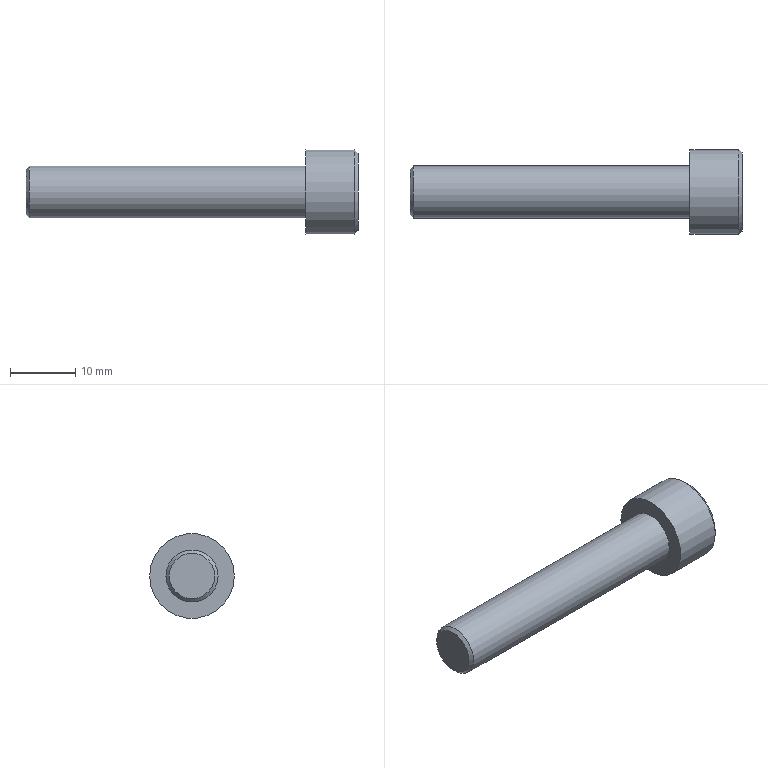Part | NX | features CHAMFER 6, BREP 2, solid 2, SUBTRACT 1 | 1 solid | 36 faces | box 51 x 13 x 13 mm | volume 3079 mm3 | plane 23 | spline 9 | cylinder 2 | cone 2 | commonest cylinder face diameters 8 x1 13 x1
STEP:
#1=CARTESIAN_POINT('',(260.,-279.45,211.002));
#2=VERTEX_POINT('',#1);
#3=CARTESIAN_POINT('',(260.,-279.625,211.545));
#4=VERTEX_POINT('',#3);
#5=CARTESIAN_POINT('',(260.,-279.45,211.002));
#6=CARTESIAN_POINT('',(260.,-279.385,211.002));
#7=CARTESIAN_POINT('',(260.,-279.327,211.016));
#8=CARTESIAN_POINT('',(260.,-279.225,211.073));
#9=CARTESIAN_POINT('',(260.,-279.185,211.113));
#10=CARTESIAN_POINT('',(260.,-279.128,211.215));
#11=CARTESIAN_POINT('',(260.,-279.114,211.272));
#12=CARTESIAN_POINT('',(260.,-279.114,211.377));
#13=CARTESIAN_POINT('',(260.,-279.121,211.418));
#14=CARTESIAN_POINT('',(260.,-279.15,211.497));
#15=CARTESIAN_POINT('',(260.,-279.171,211.531));
#16=CARTESIAN_POINT('',(260.,-279.224,211.589));
#17=CARTESIAN_POINT('',(260.,-279.256,211.611));
#18=CARTESIAN_POINT('',(260.,-279.327,211.643));
#19=CARTESIAN_POINT('',(260.,-279.366,211.651));
#20=CARTESIAN_POINT('',(260.,-279.452,211.651));
#21=CARTESIAN_POINT('',(260.,-279.491,211.642));
#22=CARTESIAN_POINT('',(260.,-279.562,211.608));
#23=CARTESIAN_POINT('',(260.,-279.595,211.581));
#24=CARTESIAN_POINT('',(260.,-279.625,211.545));
#25=B_SPLINE_CURVE_WITH_KNOTS('',3,(#5,#6,#7,#8,#9,#10,#11,#12,#13,#14,#15,#16,#17,#18,#19,#20,#21,#22,#23,#24),.UNSPECIFIED.,.F.,.F.,(4,2,2,2,2,2,2,2,2,4),(0.,0.02844,0.05688,0.08532,0.1049,0.1245,0.144,0.1636,0.184,0.2044),.UNSPECIFIED.);
#26=EDGE_CURVE('',#2,#4,#25,.T.);
#27=ORIENTED_EDGE('',*,*,#26,.F.);
#28=CARTESIAN_POINT('',(260.,-279.314,211.783));
#29=VERTEX_POINT('',#28);
#30=CARTESIAN_POINT('',(260.,-279.314,211.783));
#31=CARTESIAN_POINT('',(260.,-279.306,211.762));
#32=CARTESIAN_POINT('',(260.,-279.294,211.746));
#33=CARTESIAN_POINT('',(260.,-279.262,211.722));
#34=CARTESIAN_POINT('',(260.,-279.245,211.716));
#35=CARTESIAN_POINT('',(260.,-279.205,211.716));
#36=CARTESIAN_POINT('',(260.,-279.188,211.724));
#37=CARTESIAN_POINT('',(260.,-279.16,211.754));
#38=CARTESIAN_POINT('',(260.,-279.154,211.77));
#39=CARTESIAN_POINT('',(260.,-279.154,211.818));
#40=CARTESIAN_POINT('',(260.,-279.164,211.85));
#41=CARTESIAN_POINT('',(260.,-279.208,211.915));
#42=CARTESIAN_POINT('',(260.,-279.241,211.943));
#43=CARTESIAN_POINT('',(260.,-279.327,211.987));
#44=CARTESIAN_POINT('',(260.,-279.377,211.998));
#45=CARTESIAN_POINT('',(260.,-279.493,211.998));
#46=CARTESIAN_POINT('',(260.,-279.545,211.987));
#47=CARTESIAN_POINT('',(260.,-279.637,211.943));
#48=CARTESIAN_POINT('',(260.,-279.676,211.91));
#49=CARTESIAN_POINT('',(260.,-279.741,211.823));
#50=CARTESIAN_POINT('',(260.,-279.766,211.769));
#51=CARTESIAN_POINT('',(260.,-279.8,211.637));
#52=CARTESIAN_POINT('',(260.,-279.809,211.562));
#53=CARTESIAN_POINT('',(260.,-279.809,211.375));
#54=CARTESIAN_POINT('',(260.,-279.795,211.288));
#55=CARTESIAN_POINT('',(260.,-279.738,211.146));
#56=CARTESIAN_POINT('',(260.,-279.696,211.093));
#57=CARTESIAN_POINT('',(260.,-279.588,211.02));
#58=CARTESIAN_POINT('',(260.,-279.524,211.002));
#59=CARTESIAN_POINT('',(260.,-279.45,211.002));
#60=B_SPLINE_CURVE_WITH_KNOTS('',3,(#30,#31,#32,#33,#34,#35,#36,#37,#38,#39,#40,#41,#42,#43,#44,#45,#46,#47,#48,#49,#50,#51,#52,#53,#54,#55,#56,#57,#58,#59),.UNSPECIFIED.,.F.,.F.,(4,2,2,2,2,2,2,2,2,2,2,2,2,2,4),(0.3727,0.3977,0.4227,0.4513,0.4798,0.5272,0.5745,0.6219,0.6711,0.7203,0.7695,0.8188,0.8792,0.9396,1.),.UNSPECIFIED.);
#61=EDGE_CURVE('',#29,#2,#60,.T.);
#62=ORIENTED_EDGE('',*,*,#61,.F.);
#63=CARTESIAN_POINT('',(260.,-279.568,211.796));
#64=VERTEX_POINT('',#63);
#65=CARTESIAN_POINT('',(260.,-279.568,211.796));
#66=CARTESIAN_POINT('',(260.,-279.552,211.819));
#67=CARTESIAN_POINT('',(260.,-279.532,211.837));
#68=CARTESIAN_POINT('',(260.,-279.486,211.864));
#69=CARTESIAN_POINT('',(260.,-279.463,211.871));
#70=CARTESIAN_POINT('',(260.,-279.41,211.871));
#71=CARTESIAN_POINT('',(260.,-279.384,211.863));
#72=CARTESIAN_POINT('',(260.,-279.34,211.831));
#73=CARTESIAN_POINT('',(260.,-279.324,211.809));
#74=CARTESIAN_POINT('',(260.,-279.314,211.783));
#75=B_SPLINE_CURVE_WITH_KNOTS('',3,(#65,#66,#67,#68,#69,#70,#71,#72,#73,#74),.UNSPECIFIED.,.F.,.F.,(4,2,2,2,4),(0.2569,0.2827,0.3085,0.3406,0.3727),.UNSPECIFIED.);
#76=EDGE_CURVE('',#64,#29,#75,.T.);
#77=ORIENTED_EDGE('',*,*,#76,.F.);
#78=CARTESIAN_POINT('',(260.,-279.625,211.545));
#79=CARTESIAN_POINT('',(260.,-279.619,211.666));
#80=CARTESIAN_POINT('',(260.,-279.6,211.749));
#81=CARTESIAN_POINT('',(260.,-279.568,211.796));
#82=B_SPLINE_CURVE_WITH_KNOTS('',3,(#78,#79,#80,#81),.UNSPECIFIED.,.F.,.F.,(4,4),(0.2044,0.2569),.PIECEWISE_BEZIER_KNOTS.);
#83=EDGE_CURVE('',#4,#64,#82,.T.);
#84=ORIENTED_EDGE('',*,*,#83,.F.);
#85=EDGE_LOOP('',(#27,#62,#77,#84));
#86=FACE_BOUND('',#85,.T.);
#87=CARTESIAN_POINT('',(260.,-281.732,208.5));
#88=VERTEX_POINT('',#87);
#89=CARTESIAN_POINT('',(260.,-283.464,211.5));
#90=VERTEX_POINT('',#89);
#91=CARTESIAN_POINT('',(260.,-283.464,211.5));
#92=DIRECTION('',(0.,-0.5,0.866));
#93=VECTOR('',#92,1000.);
#94=LINE('',#91,#93);
#95=EDGE_CURVE('',#88,#90,#94,.T.);
#96=ORIENTED_EDGE('',*,*,#95,.F.);
#97=CARTESIAN_POINT('',(260.,-278.268,208.5));
#98=VERTEX_POINT('',#97);
#99=CARTESIAN_POINT('',(260.,-281.732,208.5));
#100=DIRECTION('',(0.,-1.,0.));
#101=VECTOR('',#100,1000.);
#102=LINE('',#99,#101);
#103=EDGE_CURVE('',#98,#88,#102,.T.);
#104=ORIENTED_EDGE('',*,*,#103,.F.);
#105=CARTESIAN_POINT('',(260.,-276.536,211.5));
#106=VERTEX_POINT('',#105);
#107=CARTESIAN_POINT('',(260.,-278.268,208.5));
#108=DIRECTION('',(0.,-0.5,-0.866));
#109=VECTOR('',#108,1000.);
#110=LINE('',#107,#109);
#111=EDGE_CURVE('',#106,#98,#110,.T.);
#112=ORIENTED_EDGE('',*,*,#111,.F.);
#113=CARTESIAN_POINT('',(260.,-278.268,214.5));
#114=VERTEX_POINT('',#113);
#115=CARTESIAN_POINT('',(260.,-276.536,211.5));
#116=DIRECTION('',(0.,0.5,-0.866));
#117=VECTOR('',#116,1000.);
#118=LINE('',#115,#117);
#119=EDGE_CURVE('',#114,#106,#118,.T.);
#120=ORIENTED_EDGE('',*,*,#119,.F.);
#121=CARTESIAN_POINT('',(260.,-281.732,214.5));
#122=VERTEX_POINT('',#121);
#123=CARTESIAN_POINT('',(260.,-278.268,214.5));
#124=DIRECTION('',(0.,1.,0.));
#125=VECTOR('',#124,1000.);
#126=LINE('',#123,#125);
#127=EDGE_CURVE('',#122,#114,#126,.T.);
#128=ORIENTED_EDGE('',*,*,#127,.F.);
#129=CARTESIAN_POINT('',(260.,-281.732,214.5));
#130=DIRECTION('',(0.,0.5,0.866));
#131=VECTOR('',#130,1000.);
#132=LINE('',#129,#131);
#133=EDGE_CURVE('',#90,#122,#132,.T.);
#134=ORIENTED_EDGE('',*,*,#133,.F.);
#135=EDGE_LOOP('',(#96,#104,#112,#120,#128,#134));
#136=FACE_BOUND('',#135,.T.);
#137=CARTESIAN_POINT('',(260.,-280.797,211.005));
#138=VERTEX_POINT('',#137);
#139=CARTESIAN_POINT('',(260.,-280.706,211.783));
#140=VERTEX_POINT('',#139);
#141=CARTESIAN_POINT('',(260.,-280.797,211.005));
#142=CARTESIAN_POINT('',(260.,-280.769,211.005));
#143=CARTESIAN_POINT('',(260.,-280.748,211.014));
#144=CARTESIAN_POINT('',(260.,-280.715,211.051));
#145=CARTESIAN_POINT('',(260.,-280.706,211.079));
#146=CARTESIAN_POINT('',(260.,-280.706,211.338));
#147=CARTESIAN_POINT('',(260.,-280.706,211.561));
#148=CARTESIAN_POINT('',(260.,-280.706,211.783));
#149=B_SPLINE_CURVE_WITH_KNOTS('',3,(#141,#142,#143,#144,#145,#146,#147,#148),.UNSPECIFIED.,.F.,.F.,(4,2,2,4),(0.,0.01767,0.03533,0.1418),.UNSPECIFIED.);
#150=EDGE_CURVE('',#138,#140,#149,.T.);
#151=ORIENTED_EDGE('',*,*,#150,.F.);
#152=CARTESIAN_POINT('',(260.,-280.561,211.859));
#153=VERTEX_POINT('',#152);
#154=CARTESIAN_POINT('',(260.,-280.561,211.859));
#155=CARTESIAN_POINT('',(260.,-280.571,211.898));
#156=CARTESIAN_POINT('',(260.,-280.58,211.925));
#157=CARTESIAN_POINT('',(260.,-280.596,211.96));
#158=CARTESIAN_POINT('',(260.,-280.608,211.972));
#159=CARTESIAN_POINT('',(260.,-280.641,211.985));
#160=CARTESIAN_POINT('',(260.,-280.667,211.988));
#161=CARTESIAN_POINT('',(260.,-280.724,211.988));
#162=CARTESIAN_POINT('',(260.,-280.744,211.988));
#163=CARTESIAN_POINT('',(260.,-280.802,211.988));
#164=CARTESIAN_POINT('',(260.,-280.831,211.981));
#165=CARTESIAN_POINT('',(260.,-280.875,211.951));
#166=CARTESIAN_POINT('',(260.,-280.886,211.923));
#167=CARTESIAN_POINT('',(260.,-280.886,211.626));
#168=CARTESIAN_POINT('',(260.,-280.886,211.371));
#169=CARTESIAN_POINT('',(260.,-280.886,211.079));
#170=CARTESIAN_POINT('',(260.,-280.878,211.051));
#171=CARTESIAN_POINT('',(260.,-280.845,211.014));
#172=CARTESIAN_POINT('',(260.,-280.823,211.005));
#173=CARTESIAN_POINT('',(260.,-280.797,211.005));
#174=B_SPLINE_CURVE_WITH_KNOTS('',3,(#154,#155,#156,#157,#158,#159,#160,#161,#162,#163,#164,#165,#166,#167,#168,#169,#170,#171,#172,#173),.UNSPECIFIED.,.F.,.F.,(4,2,2,2,2,2,2,2,2,4),(0.8075,0.8217,0.8358,0.85,0.8578,0.8723,0.8868,0.9743,0.9872,1.),.UNSPECIFIED.);
#175=EDGE_CURVE('',#153,#138,#174,.T.);
#176=ORIENTED_EDGE('',*,*,#175,.F.);
#177=CARTESIAN_POINT('',(260.,-280.42,211.33));
#178=VERTEX_POINT('',#177);
#179=CARTESIAN_POINT('',(260.,-280.435,211.385));
#180=DIRECTION('',(0.,-0.2564,0.9666));
#181=VECTOR('',#180,1000.);
#182=LINE('',#179,#181);
#183=EDGE_CURVE('',#178,#153,#182,.T.);
#184=ORIENTED_EDGE('',*,*,#183,.F.);
#185=CARTESIAN_POINT('',(260.,-280.28,211.859));
#186=VERTEX_POINT('',#185);
#187=CARTESIAN_POINT('',(260.,-280.35,211.593));
#188=DIRECTION('',(0.,-0.2564,-0.9666));
#189=VECTOR('',#188,1000.);
#190=LINE('',#187,#189);
#191=EDGE_CURVE('',#186,#178,#190,.T.);
#192=ORIENTED_EDGE('',*,*,#191,.F.);
#193=CARTESIAN_POINT('',(260.,-280.134,211.783));
#194=VERTEX_POINT('',#193);
#195=CARTESIAN_POINT('',(260.,-280.134,211.783));
#196=CARTESIAN_POINT('',(260.,-280.134,211.561));
#197=CARTESIAN_POINT('',(260.,-280.134,211.338));
#198=CARTESIAN_POINT('',(260.,-280.134,211.079));
#199=CARTESIAN_POINT('',(260.,-280.126,211.051));
#200=CARTESIAN_POINT('',(260.,-280.092,211.014));
#201=CARTESIAN_POINT('',(260.,-280.071,211.005));
#202=CARTESIAN_POINT('',(260.,-280.018,211.005));
#203=CARTESIAN_POINT('',(260.,-279.995,211.014));
#204=CARTESIAN_POINT('',(260.,-279.962,211.051));
#205=CARTESIAN_POINT('',(260.,-279.954,211.079));
#206=CARTESIAN_POINT('',(260.,-279.954,211.371));
#207=CARTESIAN_POINT('',(260.,-279.954,211.626));
#208=CARTESIAN_POINT('',(260.,-279.954,211.923));
#209=CARTESIAN_POINT('',(260.,-279.965,211.951));
#210=CARTESIAN_POINT('',(260.,-280.009,211.981));
#211=CARTESIAN_POINT('',(260.,-280.039,211.988));
#212=CARTESIAN_POINT('',(260.,-280.096,211.988));
#213=CARTESIAN_POINT('',(260.,-280.117,211.988));
#214=CARTESIAN_POINT('',(260.,-280.173,211.988));
#215=CARTESIAN_POINT('',(260.,-280.2,211.985));
#216=CARTESIAN_POINT('',(260.,-280.233,211.972));
#217=CARTESIAN_POINT('',(260.,-280.245,211.96));
#218=CARTESIAN_POINT('',(260.,-280.261,211.925));
#219=CARTESIAN_POINT('',(260.,-280.27,211.898));
#220=CARTESIAN_POINT('',(260.,-280.28,211.859));
#221=B_SPLINE_CURVE_WITH_KNOTS('',3,(#195,#196,#197,#198,#199,#200,#201,#202,#203,#204,#205,#206,#207,#208,#209,#210,#211,#212,#213,#214,#215,#216,#217,#218,#219,#220),.UNSPECIFIED.,.F.,.F.,(4,2,2,2,2,2,2,2,2,2,2,2,4),(0.3909,0.4624,0.4743,0.4862,0.4988,0.5115,0.599,0.6135,0.628,0.6359,0.65,0.6642,0.6783),.UNSPECIFIED.);
#222=EDGE_CURVE('',#194,#186,#221,.T.);
#223=ORIENTED_EDGE('',*,*,#222,.F.);
#224=CARTESIAN_POINT('',(260.,-280.289,211.167));
#225=VERTEX_POINT('',#224);
#226=CARTESIAN_POINT('',(260.,-280.193,211.549));
#227=DIRECTION('',(0.,0.244,0.9698));
#228=VECTOR('',#227,1000.);
#229=LINE('',#226,#228);
#230=EDGE_CURVE('',#225,#194,#229,.T.);
#231=ORIENTED_EDGE('',*,*,#230,.F.);
#232=CARTESIAN_POINT('',(260.,-280.551,211.167));
#233=VERTEX_POINT('',#232);
#234=CARTESIAN_POINT('',(260.,-280.551,211.167));
#235=CARTESIAN_POINT('',(260.,-280.546,211.147));
#236=CARTESIAN_POINT('',(260.,-280.541,211.128));
#237=CARTESIAN_POINT('',(260.,-280.531,211.09));
#238=CARTESIAN_POINT('',(260.,-280.524,211.073));
#239=CARTESIAN_POINT('',(260.,-280.506,211.043));
#240=CARTESIAN_POINT('',(260.,-280.494,211.03));
#241=CARTESIAN_POINT('',(260.,-280.462,211.01));
#242=CARTESIAN_POINT('',(260.,-280.443,211.005));
#243=CARTESIAN_POINT('',(260.,-280.39,211.005));
#244=CARTESIAN_POINT('',(260.,-280.366,211.013));
#245=CARTESIAN_POINT('',(260.,-280.332,211.044));
#246=CARTESIAN_POINT('',(260.,-280.32,211.061));
#247=CARTESIAN_POINT('',(260.,-280.307,211.098));
#248=CARTESIAN_POINT('',(260.,-280.299,211.127));
#249=CARTESIAN_POINT('',(260.,-280.289,211.167));
#250=B_SPLINE_CURVE_WITH_KNOTS('',3,(#234,#235,#236,#237,#238,#239,#240,#241,#242,#243,#244,#245,#246,#247,#248,#249),.UNSPECIFIED.,.F.,.F.,(4,2,2,2,2,2,2,4),(0.243,0.253,0.263,0.273,0.283,0.2963,0.3096,0.3228),.UNSPECIFIED.);
#251=EDGE_CURVE('',#233,#225,#250,.T.);
#252=ORIENTED_EDGE('',*,*,#251,.F.);
#253=CARTESIAN_POINT('',(260.,-280.597,211.35));
#254=DIRECTION('',(0.,0.244,-0.9698));
#255=VECTOR('',#254,1000.);
#256=LINE('',#253,#255);
#257=EDGE_CURVE('',#140,#233,#256,.T.);
#258=ORIENTED_EDGE('',*,*,#257,.F.);
#259=EDGE_LOOP('',(#151,#176,#184,#192,#223,#231,#252,#258));
#260=FACE_BOUND('',#259,.T.);
#261=CARTESIAN_POINT('',(260.,-280.,211.5));
#262=DIRECTION('',(1.,0.,0.));
#263=DIRECTION('',(0.,-1.,0.));
#264=AXIS2_PLACEMENT_3D('',#261,#262,#263);
#265=PLANE('',#264);
#266=ADVANCED_FACE('',(#86,#136,#260),#265,.T.);
#267=CARTESIAN_POINT('',(213.,-283.5,211.5));
#268=VERTEX_POINT('',#267);
#269=CARTESIAN_POINT('',(213.,-280.,211.5));
#270=DIRECTION('',(-1.,0.,0.));
#271=DIRECTION('',(0.,-1.,0.));
#272=AXIS2_PLACEMENT_3D('',#269,#270,#271);
#273=CIRCLE('',#272,3.5);
#274=EDGE_CURVE('',#268,#268,#273,.T.);
#275=ORIENTED_EDGE('',*,*,#274,.T.);
#276=EDGE_LOOP('',(#275));
#277=FACE_BOUND('',#276,.T.);
#278=CARTESIAN_POINT('',(213.,-280.,207.5));
#279=DIRECTION('',(-1.,0.,0.));
#280=DIRECTION('',(0.,1.,0.));
#281=AXIS2_PLACEMENT_3D('',#278,#279,#280);
#282=PLANE('',#281);
#283=ADVANCED_FACE('',(#277),#282,.T.);
#284=CARTESIAN_POINT('',(213.5,-284.,211.5));
#285=VERTEX_POINT('',#284);
#286=CARTESIAN_POINT('',(213.5,-280.,211.5));
#287=DIRECTION('',(1.,0.,0.));
#288=DIRECTION('',(0.,-1.,0.));
#289=AXIS2_PLACEMENT_3D('',#286,#287,#288);
#290=CIRCLE('',#289,4.);
#291=EDGE_CURVE('',#285,#285,#290,.T.);
#292=ORIENTED_EDGE('',*,*,#291,.T.);
#293=EDGE_LOOP('',(#292));
#294=FACE_BOUND('',#293,.T.);
#295=CARTESIAN_POINT('',(256.,-276.,211.5));
#296=VERTEX_POINT('',#295);
#297=CARTESIAN_POINT('',(256.,-280.,211.5));
#298=DIRECTION('',(1.,0.,0.));
#299=DIRECTION('',(0.,1.,0.));
#300=AXIS2_PLACEMENT_3D('',#297,#298,#299);
#301=CIRCLE('',#300,4.);
#302=EDGE_CURVE('',#296,#296,#301,.T.);
#303=ORIENTED_EDGE('',*,*,#302,.F.);
#304=EDGE_LOOP('',(#303));
#305=FACE_BOUND('',#304,.T.);
#306=CARTESIAN_POINT('',(265.,-280.,211.5));
#307=DIRECTION('',(1.,0.,0.));
#308=DIRECTION('',(0.,-1.,0.));
#309=AXIS2_PLACEMENT_3D('',#306,#307,#308);
#310=CYLINDRICAL_SURFACE('',#309,4.);
#311=ADVANCED_FACE('',(#294,#305),#310,.T.);
#312=ORIENTED_EDGE('',*,*,#302,.T.);
#313=EDGE_LOOP('',(#312));
#314=FACE_BOUND('',#313,.T.);
#315=CARTESIAN_POINT('',(256.,-273.5,211.5));
#316=VERTEX_POINT('',#315);
#317=CARTESIAN_POINT('',(256.,-280.,211.5));
#318=DIRECTION('',(1.,0.,0.));
#319=DIRECTION('',(0.,1.,0.));
#320=AXIS2_PLACEMENT_3D('',#317,#318,#319);
#321=CIRCLE('',#320,6.5);
#322=EDGE_CURVE('',#316,#316,#321,.T.);
#323=ORIENTED_EDGE('',*,*,#322,.F.);
#324=EDGE_LOOP('',(#323));
#325=FACE_BOUND('',#324,.T.);
#326=CARTESIAN_POINT('',(256.,-280.,205.));
#327=DIRECTION('',(-1.,0.,0.));
#328=DIRECTION('',(0.,1.,0.));
#329=AXIS2_PLACEMENT_3D('',#326,#327,#328);
#330=PLANE('',#329);
#331=ADVANCED_FACE('',(#314,#325),#330,.T.);
#332=CARTESIAN_POINT('',(263.5,-273.5,211.5));
#333=VERTEX_POINT('',#332);
#334=CARTESIAN_POINT('',(263.5,-280.,211.5));
#335=DIRECTION('',(-1.,0.,0.));
#336=DIRECTION('',(0.,1.,0.));
#337=AXIS2_PLACEMENT_3D('',#334,#335,#336);
#338=CIRCLE('',#337,6.5);
#339=EDGE_CURVE('',#333,#333,#338,.T.);
#340=ORIENTED_EDGE('',*,*,#339,.T.);
#341=EDGE_LOOP('',(#340));
#342=FACE_BOUND('',#341,.T.);
#343=ORIENTED_EDGE('',*,*,#322,.T.);
#344=EDGE_LOOP('',(#343));
#345=FACE_BOUND('',#344,.T.);
#346=CARTESIAN_POINT('',(265.,-280.,211.5));
#347=DIRECTION('',(1.,0.,0.));
#348=DIRECTION('',(0.,-1.,0.));
#349=AXIS2_PLACEMENT_3D('',#346,#347,#348);
#350=CYLINDRICAL_SURFACE('',#349,6.5);
#351=ADVANCED_FACE('',(#342,#345),#350,.T.);
#352=CARTESIAN_POINT('',(264.,-274.,211.5));
#353=VERTEX_POINT('',#352);
#354=CARTESIAN_POINT('',(264.,-280.,211.5));
#355=DIRECTION('',(1.,0.,0.));
#356=DIRECTION('',(0.,1.,0.));
#357=AXIS2_PLACEMENT_3D('',#354,#355,#356);
#358=CIRCLE('',#357,6.);
#359=EDGE_CURVE('',#353,#353,#358,.T.);
#360=ORIENTED_EDGE('',*,*,#359,.T.);
#361=EDGE_LOOP('',(#360));
#362=FACE_BOUND('',#361,.T.);
#363=CARTESIAN_POINT('',(264.,-282.309,207.5));
#364=VERTEX_POINT('',#363);
#365=CARTESIAN_POINT('',(264.,-284.619,211.5));
#366=VERTEX_POINT('',#365);
#367=CARTESIAN_POINT('',(264.,-284.33,211.));
#368=DIRECTION('',(0.,-0.5,0.866));
#369=VECTOR('',#368,1000.);
#370=LINE('',#367,#369);
#371=EDGE_CURVE('',#364,#366,#370,.T.);
#372=ORIENTED_EDGE('',*,*,#371,.T.);
#373=CARTESIAN_POINT('',(264.,-282.309,215.5));
#374=VERTEX_POINT('',#373);
#375=CARTESIAN_POINT('',(264.,-282.021,216.));
#376=DIRECTION('',(0.,0.5,0.866));
#377=VECTOR('',#376,1000.);
#378=LINE('',#375,#377);
#379=EDGE_CURVE('',#366,#374,#378,.T.);
#380=ORIENTED_EDGE('',*,*,#379,.T.);
#381=CARTESIAN_POINT('',(264.,-277.691,215.5));
#382=VERTEX_POINT('',#381);
#383=CARTESIAN_POINT('',(264.,-277.113,215.5));
#384=DIRECTION('',(0.,1.,0.));
#385=VECTOR('',#384,1000.);
#386=LINE('',#383,#385);
#387=EDGE_CURVE('',#374,#382,#386,.T.);
#388=ORIENTED_EDGE('',*,*,#387,.T.);
#389=CARTESIAN_POINT('',(264.,-275.381,211.5));
#390=VERTEX_POINT('',#389);
#391=CARTESIAN_POINT('',(264.,-275.093,211.));
#392=DIRECTION('',(0.,0.5,-0.866));
#393=VECTOR('',#392,1000.);
#394=LINE('',#391,#393);
#395=EDGE_CURVE('',#382,#390,#394,.T.);
#396=ORIENTED_EDGE('',*,*,#395,.T.);
#397=CARTESIAN_POINT('',(264.,-277.691,207.5));
#398=VERTEX_POINT('',#397);
#399=CARTESIAN_POINT('',(264.,-277.979,207.));
#400=DIRECTION('',(0.,-0.5,-0.866));
#401=VECTOR('',#400,1000.);
#402=LINE('',#399,#401);
#403=EDGE_CURVE('',#390,#398,#402,.T.);
#404=ORIENTED_EDGE('',*,*,#403,.T.);
#405=CARTESIAN_POINT('',(264.,-282.887,207.5));
#406=DIRECTION('',(0.,-1.,0.));
#407=VECTOR('',#406,1000.);
#408=LINE('',#405,#407);
#409=EDGE_CURVE('',#398,#364,#408,.T.);
#410=ORIENTED_EDGE('',*,*,#409,.T.);
#411=EDGE_LOOP('',(#372,#380,#388,#396,#404,#410));
#412=FACE_BOUND('',#411,.T.);
#413=CARTESIAN_POINT('',(264.,-280.,211.5));
#414=DIRECTION('',(1.,0.,0.));
#415=DIRECTION('',(0.,-1.,0.));
#416=AXIS2_PLACEMENT_3D('',#413,#414,#415);
#417=PLANE('',#416);
#418=ADVANCED_FACE('',(#362,#412),#417,.T.);
#419=CARTESIAN_POINT('',(263.,-283.464,211.5));
#420=VERTEX_POINT('',#419);
#421=CARTESIAN_POINT('',(260.,-283.464,211.5));
#422=DIRECTION('',(-1.,0.,0.));
#423=VECTOR('',#422,1000.);
#424=LINE('',#421,#423);
#425=EDGE_CURVE('',#420,#90,#424,.T.);
#426=ORIENTED_EDGE('',*,*,#425,.F.);
#427=CARTESIAN_POINT('',(263.,-281.732,208.5));
#428=VERTEX_POINT('',#427);
#429=CARTESIAN_POINT('',(263.,-281.732,208.5));
#430=DIRECTION('',(0.,0.5,-0.866));
#431=VECTOR('',#430,1000.);
#432=LINE('',#429,#431);
#433=EDGE_CURVE('',#420,#428,#432,.T.);
#434=ORIENTED_EDGE('',*,*,#433,.T.);
#435=CARTESIAN_POINT('',(260.,-281.732,208.5));
#436=DIRECTION('',(-1.,0.,0.));
#437=VECTOR('',#436,1000.);
#438=LINE('',#435,#437);
#439=EDGE_CURVE('',#428,#88,#438,.T.);
#440=ORIENTED_EDGE('',*,*,#439,.T.);
#441=ORIENTED_EDGE('',*,*,#95,.T.);
#442=EDGE_LOOP('',(#426,#434,#440,#441));
#443=FACE_BOUND('',#442,.T.);
#444=CARTESIAN_POINT('',(260.,-283.464,211.5));
#445=DIRECTION('',(0.,-0.866,-0.5));
#446=DIRECTION('',(0.,-0.5,0.866));
#447=AXIS2_PLACEMENT_3D('',#444,#445,#446);
#448=PLANE('',#447);
#449=ADVANCED_FACE('',(#443),#448,.F.);
#450=ORIENTED_EDGE('',*,*,#439,.F.);
#451=CARTESIAN_POINT('',(263.,-278.268,208.5));
#452=VERTEX_POINT('',#451);
#453=CARTESIAN_POINT('',(263.,-278.268,208.5));
#454=DIRECTION('',(0.,1.,0.));
#455=VECTOR('',#454,1000.);
#456=LINE('',#453,#455);
#457=EDGE_CURVE('',#428,#452,#456,.T.);
#458=ORIENTED_EDGE('',*,*,#457,.T.);
#459=CARTESIAN_POINT('',(260.,-278.268,208.5));
#460=DIRECTION('',(-1.,0.,0.));
#461=VECTOR('',#460,1000.);
#462=LINE('',#459,#461);
#463=EDGE_CURVE('',#452,#98,#462,.T.);
#464=ORIENTED_EDGE('',*,*,#463,.T.);
#465=ORIENTED_EDGE('',*,*,#103,.T.);
#466=EDGE_LOOP('',(#450,#458,#464,#465));
#467=FACE_BOUND('',#466,.T.);
#468=CARTESIAN_POINT('',(260.,-281.732,208.5));
#469=DIRECTION('',(0.,0.,-1.));
#470=DIRECTION('',(0.,-1.,0.));
#471=AXIS2_PLACEMENT_3D('',#468,#469,#470);
#472=PLANE('',#471);
#473=ADVANCED_FACE('',(#467),#472,.F.);
#474=ORIENTED_EDGE('',*,*,#463,.F.);
#475=CARTESIAN_POINT('',(263.,-276.536,211.5));
#476=VERTEX_POINT('',#475);
#477=CARTESIAN_POINT('',(263.,-276.536,211.5));
#478=DIRECTION('',(0.,0.5,0.866));
#479=VECTOR('',#478,1000.);
#480=LINE('',#477,#479);
#481=EDGE_CURVE('',#452,#476,#480,.T.);
#482=ORIENTED_EDGE('',*,*,#481,.T.);
#483=CARTESIAN_POINT('',(260.,-276.536,211.5));
#484=DIRECTION('',(-1.,0.,0.));
#485=VECTOR('',#484,1000.);
#486=LINE('',#483,#485);
#487=EDGE_CURVE('',#476,#106,#486,.T.);
#488=ORIENTED_EDGE('',*,*,#487,.T.);
#489=ORIENTED_EDGE('',*,*,#111,.T.);
#490=EDGE_LOOP('',(#474,#482,#488,#489));
#491=FACE_BOUND('',#490,.T.);
#492=CARTESIAN_POINT('',(260.,-278.268,208.5));
#493=DIRECTION('',(0.,0.866,-0.5));
#494=DIRECTION('',(0.,-0.5,-0.866));
#495=AXIS2_PLACEMENT_3D('',#492,#493,#494);
#496=PLANE('',#495);
#497=ADVANCED_FACE('',(#491),#496,.F.);
#498=ORIENTED_EDGE('',*,*,#487,.F.);
#499=CARTESIAN_POINT('',(263.,-278.268,214.5));
#500=VERTEX_POINT('',#499);
#501=CARTESIAN_POINT('',(263.,-278.268,214.5));
#502=DIRECTION('',(0.,-0.5,0.866));
#503=VECTOR('',#502,1000.);
#504=LINE('',#501,#503);
#505=EDGE_CURVE('',#476,#500,#504,.T.);
#506=ORIENTED_EDGE('',*,*,#505,.T.);
#507=CARTESIAN_POINT('',(260.,-278.268,214.5));
#508=DIRECTION('',(-1.,0.,0.));
#509=VECTOR('',#508,1000.);
#510=LINE('',#507,#509);
#511=EDGE_CURVE('',#500,#114,#510,.T.);
#512=ORIENTED_EDGE('',*,*,#511,.T.);
#513=ORIENTED_EDGE('',*,*,#119,.T.);
#514=EDGE_LOOP('',(#498,#506,#512,#513));
#515=FACE_BOUND('',#514,.T.);
#516=CARTESIAN_POINT('',(260.,-276.536,211.5));
#517=DIRECTION('',(0.,0.866,0.5));
#518=DIRECTION('',(0.,0.5,-0.866));
#519=AXIS2_PLACEMENT_3D('',#516,#517,#518);
#520=PLANE('',#519);
#521=ADVANCED_FACE('',(#515),#520,.F.);
#522=ORIENTED_EDGE('',*,*,#511,.F.);
#523=CARTESIAN_POINT('',(263.,-281.732,214.5));
#524=VERTEX_POINT('',#523);
#525=CARTESIAN_POINT('',(263.,-281.732,214.5));
#526=DIRECTION('',(0.,-1.,0.));
#527=VECTOR('',#526,1000.);
#528=LINE('',#525,#527);
#529=EDGE_CURVE('',#500,#524,#528,.T.);
#530=ORIENTED_EDGE('',*,*,#529,.T.);
#531=CARTESIAN_POINT('',(260.,-281.732,214.5));
#532=DIRECTION('',(-1.,0.,0.));
#533=VECTOR('',#532,1000.);
#534=LINE('',#531,#533);
#535=EDGE_CURVE('',#524,#122,#534,.T.);
#536=ORIENTED_EDGE('',*,*,#535,.T.);
#537=ORIENTED_EDGE('',*,*,#127,.T.);
#538=EDGE_LOOP('',(#522,#530,#536,#537));
#539=FACE_BOUND('',#538,.T.);
#540=CARTESIAN_POINT('',(260.,-278.268,214.5));
#541=DIRECTION('',(0.,0.,1.));
#542=DIRECTION('',(-1.,0.,0.));
#543=AXIS2_PLACEMENT_3D('',#540,#541,#542);
#544=PLANE('',#543);
#545=ADVANCED_FACE('',(#539),#544,.F.);
#546=ORIENTED_EDGE('',*,*,#535,.F.);
#547=CARTESIAN_POINT('',(263.,-284.041,210.5));
#548=DIRECTION('',(0.,-0.5,-0.866));
#549=VECTOR('',#548,1000.);
#550=LINE('',#547,#549);
#551=EDGE_CURVE('',#524,#420,#550,.T.);
#552=ORIENTED_EDGE('',*,*,#551,.T.);
#553=ORIENTED_EDGE('',*,*,#425,.T.);
#554=ORIENTED_EDGE('',*,*,#133,.T.);
#555=EDGE_LOOP('',(#546,#552,#553,#554));
#556=FACE_BOUND('',#555,.T.);
#557=CARTESIAN_POINT('',(260.,-281.732,214.5));
#558=DIRECTION('',(0.,-0.866,0.5));
#559=DIRECTION('',(0.,0.5,0.866));
#560=AXIS2_PLACEMENT_3D('',#557,#558,#559);
#561=PLANE('',#560);
#562=ADVANCED_FACE('',(#556),#561,.F.);
#563=ORIENTED_EDGE('',*,*,#274,.F.);
#564=EDGE_LOOP('',(#563));
#565=FACE_BOUND('',#564,.T.);
#566=ORIENTED_EDGE('',*,*,#291,.F.);
#567=EDGE_LOOP('',(#566));
#568=FACE_BOUND('',#567,.T.);
#569=CARTESIAN_POINT('',(213.5,-280.,211.5));
#570=DIRECTION('',(1.,0.,0.));
#571=DIRECTION('',(0.,-1.,0.));
#572=AXIS2_PLACEMENT_3D('',#569,#570,#571);
#573=CONICAL_SURFACE('',#572,4.,0.7854);
#574=ADVANCED_FACE('',(#565,#568),#573,.T.);
#575=ORIENTED_EDGE('',*,*,#339,.F.);
#576=EDGE_LOOP('',(#575));
#577=FACE_BOUND('',#576,.T.);
#578=ORIENTED_EDGE('',*,*,#359,.F.);
#579=EDGE_LOOP('',(#578));
#580=FACE_BOUND('',#579,.T.);
#581=CARTESIAN_POINT('',(264.,-280.,211.5));
#582=DIRECTION('',(-1.,0.,0.));
#583=DIRECTION('',(0.,1.,0.));
#584=AXIS2_PLACEMENT_3D('',#581,#582,#583);
#585=CONICAL_SURFACE('',#584,6.,0.7854);
#586=ADVANCED_FACE('',(#577,#580),#585,.T.);
#587=ORIENTED_EDGE('',*,*,#150,.T.);
#588=CARTESIAN_POINT('',(259.8,-280.706,211.783));
#589=VERTEX_POINT('',#588);
#590=CARTESIAN_POINT('',(259.8,-280.706,211.783));
#591=DIRECTION('',(1.,0.,0.));
#592=VECTOR('',#591,1000.);
#593=LINE('',#590,#592);
#594=EDGE_CURVE('',#140,#589,#593,.F.);
#595=ORIENTED_EDGE('',*,*,#594,.T.);
#596=CARTESIAN_POINT('',(259.8,-280.797,211.005));
#597=VERTEX_POINT('',#596);
#598=CARTESIAN_POINT('',(259.8,-280.797,211.005));
#599=CARTESIAN_POINT('',(259.8,-280.769,211.005));
#600=CARTESIAN_POINT('',(259.8,-280.748,211.014));
#601=CARTESIAN_POINT('',(259.8,-280.715,211.051));
#602=CARTESIAN_POINT('',(259.8,-280.706,211.079));
#603=CARTESIAN_POINT('',(259.8,-280.706,211.338));
#604=CARTESIAN_POINT('',(259.8,-280.706,211.561));
#605=CARTESIAN_POINT('',(259.8,-280.706,211.783));
#606=B_SPLINE_CURVE_WITH_KNOTS('',3,(#598,#599,#600,#601,#602,#603,#604,#605),.UNSPECIFIED.,.F.,.F.,(4,2,2,4),(0.,0.01767,0.03533,0.1418),.UNSPECIFIED.);
#607=EDGE_CURVE('',#589,#597,#606,.F.);
#608=ORIENTED_EDGE('',*,*,#607,.T.);
#609=CARTESIAN_POINT('',(259.8,-280.797,211.005));
#610=DIRECTION('',(1.,0.,0.));
#611=VECTOR('',#610,1000.);
#612=LINE('',#609,#611);
#613=EDGE_CURVE('',#138,#597,#612,.F.);
#614=ORIENTED_EDGE('',*,*,#613,.F.);
#615=EDGE_LOOP('',(#587,#595,#608,#614));
#616=FACE_BOUND('',#615,.T.);
#617=CARTESIAN_POINT('',(259.8,-280.797,211.005));
#618=CARTESIAN_POINT('',(260.,-280.797,211.005));
#619=CARTESIAN_POINT('',(259.8,-280.687,211.005));
#620=CARTESIAN_POINT('',(260.,-280.687,211.005));
#621=CARTESIAN_POINT('',(259.8,-280.716,211.357));
#622=CARTESIAN_POINT('',(260.,-280.716,211.357));
#623=CARTESIAN_POINT('',(259.8,-280.706,211.635));
#624=CARTESIAN_POINT('',(260.,-280.706,211.635));
#625=CARTESIAN_POINT('',(259.8,-280.706,211.783));
#626=CARTESIAN_POINT('',(260.,-280.706,211.783));
#627=B_SPLINE_SURFACE_WITH_KNOTS('',3,1,((#617,#618),(#619,#620),(#621,#622),(#623,#624),(#625,#626)),.SURF_OF_LINEAR_EXTRUSION.,.F.,.F.,.F.,(4,1,4),(2,2),(0.,0.07088,0.1418),(0.,1.),.UNSPECIFIED.);
#628=ADVANCED_FACE('',(#616),#627,.F.);
#629=ORIENTED_EDGE('',*,*,#257,.T.);
#630=CARTESIAN_POINT('',(259.8,-280.551,211.167));
#631=VERTEX_POINT('',#630);
#632=CARTESIAN_POINT('',(259.8,-280.551,211.167));
#633=DIRECTION('',(1.,0.,0.));
#634=VECTOR('',#633,1000.);
#635=LINE('',#632,#634);
#636=EDGE_CURVE('',#233,#631,#635,.F.);
#637=ORIENTED_EDGE('',*,*,#636,.T.);
#638=CARTESIAN_POINT('',(259.8,-280.706,211.783));
#639=CARTESIAN_POINT('',(259.8,-280.655,211.578));
#640=CARTESIAN_POINT('',(259.8,-280.603,211.373));
#641=CARTESIAN_POINT('',(259.8,-280.551,211.167));
#642=B_SPLINE_CURVE_WITH_KNOTS('',3,(#638,#639,#640,#641),.UNSPECIFIED.,.F.,.F.,(4,4),(0.1418,0.243),.PIECEWISE_BEZIER_KNOTS.);
#643=EDGE_CURVE('',#631,#589,#642,.F.);
#644=ORIENTED_EDGE('',*,*,#643,.T.);
#645=ORIENTED_EDGE('',*,*,#594,.F.);
#646=EDGE_LOOP('',(#629,#637,#644,#645));
#647=FACE_BOUND('',#646,.T.);
#648=CARTESIAN_POINT('',(259.8,-280.706,211.783));
#649=DIRECTION('',(0.,-0.9698,-0.244));
#650=DIRECTION('',(0.,0.244,-0.9698));
#651=AXIS2_PLACEMENT_3D('',#648,#649,#650);
#652=PLANE('',#651);
#653=ADVANCED_FACE('',(#647),#652,.F.);
#654=ORIENTED_EDGE('',*,*,#251,.T.);
#655=CARTESIAN_POINT('',(259.8,-280.289,211.167));
#656=VERTEX_POINT('',#655);
#657=CARTESIAN_POINT('',(259.8,-280.289,211.167));
#658=DIRECTION('',(1.,0.,0.));
#659=VECTOR('',#658,1000.);
#660=LINE('',#657,#659);
#661=EDGE_CURVE('',#225,#656,#660,.F.);
#662=ORIENTED_EDGE('',*,*,#661,.T.);
#663=CARTESIAN_POINT('',(259.8,-280.551,211.167));
#664=CARTESIAN_POINT('',(259.8,-280.546,211.147));
#665=CARTESIAN_POINT('',(259.8,-280.541,211.128));
#666=CARTESIAN_POINT('',(259.8,-280.531,211.09));
#667=CARTESIAN_POINT('',(259.8,-280.524,211.073));
#668=CARTESIAN_POINT('',(259.8,-280.506,211.043));
#669=CARTESIAN_POINT('',(259.8,-280.494,211.03));
#670=CARTESIAN_POINT('',(259.8,-280.462,211.01));
#671=CARTESIAN_POINT('',(259.8,-280.443,211.005));
#672=CARTESIAN_POINT('',(259.8,-280.39,211.005));
#673=CARTESIAN_POINT('',(259.8,-280.366,211.013));
#674=CARTESIAN_POINT('',(259.8,-280.332,211.044));
#675=CARTESIAN_POINT('',(259.8,-280.32,211.061));
#676=CARTESIAN_POINT('',(259.8,-280.307,211.098));
#677=CARTESIAN_POINT('',(259.8,-280.299,211.127));
#678=CARTESIAN_POINT('',(259.8,-280.289,211.167));
#679=B_SPLINE_CURVE_WITH_KNOTS('',3,(#663,#664,#665,#666,#667,#668,#669,#670,#671,#672,#673,#674,#675,#676,#677,#678),.UNSPECIFIED.,.F.,.F.,(4,2,2,2,2,2,2,4),(0.243,0.253,0.263,0.273,0.283,0.2963,0.3096,0.3228),.UNSPECIFIED.);
#680=EDGE_CURVE('',#656,#631,#679,.F.);
#681=ORIENTED_EDGE('',*,*,#680,.T.);
#682=ORIENTED_EDGE('',*,*,#636,.F.);
#683=EDGE_LOOP('',(#654,#662,#681,#682));
#684=FACE_BOUND('',#683,.T.);
#685=CARTESIAN_POINT('',(259.8,-280.551,211.167));
#686=CARTESIAN_POINT('',(260.,-280.551,211.167));
#687=CARTESIAN_POINT('',(259.8,-280.509,211.006));
#688=CARTESIAN_POINT('',(260.,-280.509,211.006));
#689=CARTESIAN_POINT('',(259.8,-280.35,210.927));
#690=CARTESIAN_POINT('',(260.,-280.35,210.927));
#691=CARTESIAN_POINT('',(259.8,-280.289,211.167));
#692=CARTESIAN_POINT('',(260.,-280.289,211.167));
#693=B_SPLINE_SURFACE_WITH_KNOTS('',3,1,((#685,#686),(#687,#688),(#689,#690),(#691,#692)),.SURF_OF_LINEAR_EXTRUSION.,.F.,.F.,.F.,(4,4),(2,2),(0.243,0.3228),(0.,1.),.PIECEWISE_BEZIER_KNOTS.);
#694=ADVANCED_FACE('',(#684),#693,.F.);
#695=ORIENTED_EDGE('',*,*,#230,.T.);
#696=CARTESIAN_POINT('',(259.8,-280.134,211.783));
#697=VERTEX_POINT('',#696);
#698=CARTESIAN_POINT('',(259.8,-280.134,211.783));
#699=DIRECTION('',(1.,0.,0.));
#700=VECTOR('',#699,1000.);
#701=LINE('',#698,#700);
#702=EDGE_CURVE('',#194,#697,#701,.F.);
#703=ORIENTED_EDGE('',*,*,#702,.T.);
#704=CARTESIAN_POINT('',(259.8,-280.289,211.167));
#705=CARTESIAN_POINT('',(259.8,-280.237,211.373));
#706=CARTESIAN_POINT('',(259.8,-280.186,211.578));
#707=CARTESIAN_POINT('',(259.8,-280.134,211.783));
#708=B_SPLINE_CURVE_WITH_KNOTS('',3,(#704,#705,#706,#707),.UNSPECIFIED.,.F.,.F.,(4,4),(0.3228,0.3909),.PIECEWISE_BEZIER_KNOTS.);
#709=EDGE_CURVE('',#697,#656,#708,.F.);
#710=ORIENTED_EDGE('',*,*,#709,.T.);
#711=ORIENTED_EDGE('',*,*,#661,.F.);
#712=EDGE_LOOP('',(#695,#703,#710,#711));
#713=FACE_BOUND('',#712,.T.);
#714=CARTESIAN_POINT('',(259.8,-280.289,211.167));
#715=DIRECTION('',(0.,0.9698,-0.244));
#716=DIRECTION('',(0.,0.244,0.9698));
#717=AXIS2_PLACEMENT_3D('',#714,#715,#716);
#718=PLANE('',#717);
#719=ADVANCED_FACE('',(#713),#718,.F.);
#720=ORIENTED_EDGE('',*,*,#222,.T.);
#721=CARTESIAN_POINT('',(259.8,-280.28,211.859));
#722=VERTEX_POINT('',#721);
#723=CARTESIAN_POINT('',(259.8,-280.28,211.859));
#724=DIRECTION('',(1.,0.,0.));
#725=VECTOR('',#724,1000.);
#726=LINE('',#723,#725);
#727=EDGE_CURVE('',#186,#722,#726,.F.);
#728=ORIENTED_EDGE('',*,*,#727,.T.);
#729=CARTESIAN_POINT('',(259.8,-280.134,211.783));
#730=CARTESIAN_POINT('',(259.8,-280.134,211.561));
#731=CARTESIAN_POINT('',(259.8,-280.134,211.338));
#732=CARTESIAN_POINT('',(259.8,-280.134,211.079));
#733=CARTESIAN_POINT('',(259.8,-280.126,211.051));
#734=CARTESIAN_POINT('',(259.8,-280.092,211.014));
#735=CARTESIAN_POINT('',(259.8,-280.071,211.005));
#736=CARTESIAN_POINT('',(259.8,-280.018,211.005));
#737=CARTESIAN_POINT('',(259.8,-279.995,211.014));
#738=CARTESIAN_POINT('',(259.8,-279.962,211.051));
#739=CARTESIAN_POINT('',(259.8,-279.954,211.079));
#740=CARTESIAN_POINT('',(259.8,-279.954,211.371));
#741=CARTESIAN_POINT('',(259.8,-279.954,211.626));
#742=CARTESIAN_POINT('',(259.8,-279.954,211.923));
#743=CARTESIAN_POINT('',(259.8,-279.965,211.951));
#744=CARTESIAN_POINT('',(259.8,-280.009,211.981));
#745=CARTESIAN_POINT('',(259.8,-280.039,211.988));
#746=CARTESIAN_POINT('',(259.8,-280.096,211.988));
#747=CARTESIAN_POINT('',(259.8,-280.117,211.988));
#748=CARTESIAN_POINT('',(259.8,-280.173,211.988));
#749=CARTESIAN_POINT('',(259.8,-280.2,211.985));
#750=CARTESIAN_POINT('',(259.8,-280.233,211.972));
#751=CARTESIAN_POINT('',(259.8,-280.245,211.96));
#752=CARTESIAN_POINT('',(259.8,-280.261,211.925));
#753=CARTESIAN_POINT('',(259.8,-280.27,211.898));
#754=CARTESIAN_POINT('',(259.8,-280.28,211.859));
#755=B_SPLINE_CURVE_WITH_KNOTS('',3,(#729,#730,#731,#732,#733,#734,#735,#736,#737,#738,#739,#740,#741,#742,#743,#744,#745,#746,#747,#748,#749,#750,#751,#752,#753,#754),.UNSPECIFIED.,.F.,.F.,(4,2,2,2,2,2,2,2,2,2,2,2,4),(0.3909,0.4624,0.4743,0.4862,0.4988,0.5115,0.599,0.6135,0.628,0.6359,0.65,0.6642,0.6783),.UNSPECIFIED.);
#756=EDGE_CURVE('',#722,#697,#755,.F.);
#757=ORIENTED_EDGE('',*,*,#756,.T.);
#758=ORIENTED_EDGE('',*,*,#702,.F.);
#759=EDGE_LOOP('',(#720,#728,#757,#758));
#760=FACE_BOUND('',#759,.T.);
#761=CARTESIAN_POINT('',(259.8,-280.134,211.783));
#762=CARTESIAN_POINT('',(260.,-280.134,211.783));
#763=CARTESIAN_POINT('',(259.8,-280.134,211.671));
#764=CARTESIAN_POINT('',(260.,-280.134,211.671));
#765=CARTESIAN_POINT('',(259.8,-280.119,211.461));
#766=CARTESIAN_POINT('',(260.,-280.119,211.461));
#767=CARTESIAN_POINT('',(259.8,-280.188,211.067));
#768=CARTESIAN_POINT('',(260.,-280.188,211.067));
#769=CARTESIAN_POINT('',(259.8,-279.933,210.947));
#770=CARTESIAN_POINT('',(260.,-279.933,210.947));
#771=CARTESIAN_POINT('',(259.8,-279.956,211.336));
#772=CARTESIAN_POINT('',(260.,-279.956,211.336));
#773=CARTESIAN_POINT('',(259.8,-279.969,211.613));
#774=CARTESIAN_POINT('',(260.,-279.969,211.613));
#775=CARTESIAN_POINT('',(259.8,-279.894,212.));
#776=CARTESIAN_POINT('',(260.,-279.894,212.));
#777=CARTESIAN_POINT('',(259.8,-280.231,211.994));
#778=CARTESIAN_POINT('',(260.,-280.231,211.994));
#779=CARTESIAN_POINT('',(259.8,-280.254,211.957));
#780=CARTESIAN_POINT('',(260.,-280.254,211.957));
#781=CARTESIAN_POINT('',(259.8,-280.28,211.859));
#782=CARTESIAN_POINT('',(260.,-280.28,211.859));
#783=B_SPLINE_SURFACE_WITH_KNOTS('',3,1,((#761,#762),(#763,#764),(#765,#766),(#767,#768),(#769,#770),(#771,#772),(#773,#774),(#775,#776),(#777,#778),(#779,#780),(#781,#782)),.SURF_OF_LINEAR_EXTRUSION.,.F.,.F.,.F.,(4,1,1,1,1,1,1,1,4),(2,2),(0.3909,0.4268,0.4627,0.4987,0.5346,0.5705,0.6065,0.6424,0.6783),(0.,1.),.UNSPECIFIED.);
#784=ADVANCED_FACE('',(#760),#783,.F.);
#785=ORIENTED_EDGE('',*,*,#191,.T.);
#786=CARTESIAN_POINT('',(259.8,-280.42,211.33));
#787=VERTEX_POINT('',#786);
#788=CARTESIAN_POINT('',(259.8,-280.42,211.33));
#789=DIRECTION('',(1.,0.,0.));
#790=VECTOR('',#789,1000.);
#791=LINE('',#788,#790);
#792=EDGE_CURVE('',#178,#787,#791,.F.);
#793=ORIENTED_EDGE('',*,*,#792,.T.);
#794=CARTESIAN_POINT('',(259.8,-280.28,211.859));
#795=CARTESIAN_POINT('',(259.8,-280.327,211.682));
#796=CARTESIAN_POINT('',(259.8,-280.373,211.506));
#797=CARTESIAN_POINT('',(259.8,-280.42,211.33));
#798=B_SPLINE_CURVE_WITH_KNOTS('',3,(#794,#795,#796,#797),.UNSPECIFIED.,.F.,.F.,(4,4),(0.6783,0.7429),.PIECEWISE_BEZIER_KNOTS.);
#799=EDGE_CURVE('',#787,#722,#798,.F.);
#800=ORIENTED_EDGE('',*,*,#799,.T.);
#801=ORIENTED_EDGE('',*,*,#727,.F.);
#802=EDGE_LOOP('',(#785,#793,#800,#801));
#803=FACE_BOUND('',#802,.T.);
#804=CARTESIAN_POINT('',(259.8,-280.28,211.859));
#805=DIRECTION('',(0.,-0.9666,0.2564));
#806=DIRECTION('',(0.,-0.2564,-0.9666));
#807=AXIS2_PLACEMENT_3D('',#804,#805,#806);
#808=PLANE('',#807);
#809=ADVANCED_FACE('',(#803),#808,.F.);
#810=ORIENTED_EDGE('',*,*,#183,.T.);
#811=CARTESIAN_POINT('',(259.8,-280.561,211.859));
#812=VERTEX_POINT('',#811);
#813=CARTESIAN_POINT('',(259.8,-280.561,211.859));
#814=DIRECTION('',(1.,0.,0.));
#815=VECTOR('',#814,1000.);
#816=LINE('',#813,#815);
#817=EDGE_CURVE('',#153,#812,#816,.F.);
#818=ORIENTED_EDGE('',*,*,#817,.T.);
#819=CARTESIAN_POINT('',(259.8,-280.42,211.33));
#820=CARTESIAN_POINT('',(259.8,-280.467,211.506));
#821=CARTESIAN_POINT('',(259.8,-280.514,211.682));
#822=CARTESIAN_POINT('',(259.8,-280.561,211.859));
#823=B_SPLINE_CURVE_WITH_KNOTS('',3,(#819,#820,#821,#822),.UNSPECIFIED.,.F.,.F.,(4,4),(0.7429,0.8075),.PIECEWISE_BEZIER_KNOTS.);
#824=EDGE_CURVE('',#812,#787,#823,.F.);
#825=ORIENTED_EDGE('',*,*,#824,.T.);
#826=ORIENTED_EDGE('',*,*,#792,.F.);
#827=EDGE_LOOP('',(#810,#818,#825,#826));
#828=FACE_BOUND('',#827,.T.);
#829=CARTESIAN_POINT('',(259.8,-280.42,211.33));
#830=DIRECTION('',(0.,0.9666,0.2564));
#831=DIRECTION('',(0.,-0.2564,0.9666));
#832=AXIS2_PLACEMENT_3D('',#829,#830,#831);
#833=PLANE('',#832);
#834=ADVANCED_FACE('',(#828),#833,.F.);
#835=ORIENTED_EDGE('',*,*,#175,.T.);
#836=ORIENTED_EDGE('',*,*,#613,.T.);
#837=CARTESIAN_POINT('',(259.8,-280.561,211.859));
#838=CARTESIAN_POINT('',(259.8,-280.571,211.898));
#839=CARTESIAN_POINT('',(259.8,-280.58,211.925));
#840=CARTESIAN_POINT('',(259.8,-280.596,211.96));
#841=CARTESIAN_POINT('',(259.8,-280.608,211.972));
#842=CARTESIAN_POINT('',(259.8,-280.641,211.985));
#843=CARTESIAN_POINT('',(259.8,-280.667,211.988));
#844=CARTESIAN_POINT('',(259.8,-280.724,211.988));
#845=CARTESIAN_POINT('',(259.8,-280.744,211.988));
#846=CARTESIAN_POINT('',(259.8,-280.802,211.988));
#847=CARTESIAN_POINT('',(259.8,-280.831,211.981));
#848=CARTESIAN_POINT('',(259.8,-280.875,211.951));
#849=CARTESIAN_POINT('',(259.8,-280.886,211.923));
#850=CARTESIAN_POINT('',(259.8,-280.886,211.626));
#851=CARTESIAN_POINT('',(259.8,-280.886,211.371));
#852=CARTESIAN_POINT('',(259.8,-280.886,211.079));
#853=CARTESIAN_POINT('',(259.8,-280.878,211.051));
#854=CARTESIAN_POINT('',(259.8,-280.845,211.014));
#855=CARTESIAN_POINT('',(259.8,-280.823,211.005));
#856=CARTESIAN_POINT('',(259.8,-280.797,211.005));
#857=B_SPLINE_CURVE_WITH_KNOTS('',3,(#837,#838,#839,#840,#841,#842,#843,#844,#845,#846,#847,#848,#849,#850,#851,#852,#853,#854,#855,#856),.UNSPECIFIED.,.F.,.F.,(4,2,2,2,2,2,2,2,2,4),(0.8075,0.8217,0.8358,0.85,0.8578,0.8723,0.8868,0.9743,0.9872,1.),.UNSPECIFIED.);
#858=EDGE_CURVE('',#597,#812,#857,.F.);
#859=ORIENTED_EDGE('',*,*,#858,.T.);
#860=ORIENTED_EDGE('',*,*,#817,.F.);
#861=EDGE_LOOP('',(#835,#836,#859,#860));
#862=FACE_BOUND('',#861,.T.);
#863=CARTESIAN_POINT('',(259.8,-280.561,211.859));
#864=CARTESIAN_POINT('',(260.,-280.561,211.859));
#865=CARTESIAN_POINT('',(259.8,-280.578,211.925));
#866=CARTESIAN_POINT('',(260.,-280.578,211.925));
#867=CARTESIAN_POINT('',(259.8,-280.586,211.984));
#868=CARTESIAN_POINT('',(260.,-280.586,211.984));
#869=CARTESIAN_POINT('',(259.8,-280.747,211.994));
#870=CARTESIAN_POINT('',(260.,-280.747,211.994));
#871=CARTESIAN_POINT('',(259.8,-280.91,211.969));
#872=CARTESIAN_POINT('',(260.,-280.91,211.969));
#873=CARTESIAN_POINT('',(259.8,-280.873,211.646));
#874=CARTESIAN_POINT('',(260.,-280.873,211.646));
#875=CARTESIAN_POINT('',(259.8,-280.887,211.33));
#876=CARTESIAN_POINT('',(260.,-280.887,211.33));
#877=CARTESIAN_POINT('',(259.8,-280.896,211.005));
#878=CARTESIAN_POINT('',(260.,-280.896,211.005));
#879=CARTESIAN_POINT('',(259.8,-280.797,211.005));
#880=CARTESIAN_POINT('',(260.,-280.797,211.005));
#881=B_SPLINE_SURFACE_WITH_KNOTS('',3,1,((#863,#864),(#865,#866),(#867,#868),(#869,#870),(#871,#872),(#873,#874),(#875,#876),(#877,#878),(#879,#880)),.SURF_OF_LINEAR_EXTRUSION.,.F.,.F.,.F.,(4,1,1,1,1,1,4),(2,2),(0.8075,0.8316,0.8557,0.8797,0.9038,0.9519,1.),(0.,1.),.UNSPECIFIED.);
#882=ADVANCED_FACE('',(#862),#881,.F.);
#883=ORIENTED_EDGE('',*,*,#607,.F.);
#884=ORIENTED_EDGE('',*,*,#643,.F.);
#885=ORIENTED_EDGE('',*,*,#680,.F.);
#886=ORIENTED_EDGE('',*,*,#709,.F.);
#887=ORIENTED_EDGE('',*,*,#756,.F.);
#888=ORIENTED_EDGE('',*,*,#799,.F.);
#889=ORIENTED_EDGE('',*,*,#824,.F.);
#890=ORIENTED_EDGE('',*,*,#858,.F.);
#891=EDGE_LOOP('',(#883,#884,#885,#886,#887,#888,#889,#890));
#892=FACE_BOUND('',#891,.T.);
#893=CARTESIAN_POINT('',(259.8,-280.706,211.339));
#894=DIRECTION('',(-1.,0.,0.));
#895=DIRECTION('',(0.,0.,1.));
#896=AXIS2_PLACEMENT_3D('',#893,#894,#895);
#897=PLANE('',#896);
#898=ADVANCED_FACE('',(#892),#897,.F.);
#899=ORIENTED_EDGE('',*,*,#26,.T.);
#900=CARTESIAN_POINT('',(259.8,-279.625,211.545));
#901=VERTEX_POINT('',#900);
#902=CARTESIAN_POINT('',(259.8,-279.625,211.545));
#903=DIRECTION('',(1.,0.,0.));
#904=VECTOR('',#903,1000.);
#905=LINE('',#902,#904);
#906=EDGE_CURVE('',#4,#901,#905,.F.);
#907=ORIENTED_EDGE('',*,*,#906,.T.);
#908=CARTESIAN_POINT('',(259.8,-279.45,211.002));
#909=VERTEX_POINT('',#908);
#910=CARTESIAN_POINT('',(259.8,-279.45,211.002));
#911=CARTESIAN_POINT('',(259.8,-279.385,211.002));
#912=CARTESIAN_POINT('',(259.8,-279.327,211.016));
#913=CARTESIAN_POINT('',(259.8,-279.225,211.073));
#914=CARTESIAN_POINT('',(259.8,-279.185,211.113));
#915=CARTESIAN_POINT('',(259.8,-279.128,211.215));
#916=CARTESIAN_POINT('',(259.8,-279.114,211.272));
#917=CARTESIAN_POINT('',(259.8,-279.114,211.377));
#918=CARTESIAN_POINT('',(259.8,-279.121,211.418));
#919=CARTESIAN_POINT('',(259.8,-279.15,211.497));
#920=CARTESIAN_POINT('',(259.8,-279.171,211.531));
#921=CARTESIAN_POINT('',(259.8,-279.224,211.589));
#922=CARTESIAN_POINT('',(259.8,-279.256,211.611));
#923=CARTESIAN_POINT('',(259.8,-279.327,211.643));
#924=CARTESIAN_POINT('',(259.8,-279.366,211.651));
#925=CARTESIAN_POINT('',(259.8,-279.452,211.651));
#926=CARTESIAN_POINT('',(259.8,-279.491,211.642));
#927=CARTESIAN_POINT('',(259.8,-279.562,211.608));
#928=CARTESIAN_POINT('',(259.8,-279.595,211.581));
#929=CARTESIAN_POINT('',(259.8,-279.625,211.545));
#930=B_SPLINE_CURVE_WITH_KNOTS('',3,(#910,#911,#912,#913,#914,#915,#916,#917,#918,#919,#920,#921,#922,#923,#924,#925,#926,#927,#928,#929),.UNSPECIFIED.,.F.,.F.,(4,2,2,2,2,2,2,2,2,4),(0.,0.02844,0.05688,0.08532,0.1049,0.1245,0.144,0.1636,0.184,0.2044),.UNSPECIFIED.);
#931=EDGE_CURVE('',#901,#909,#930,.F.);
#932=ORIENTED_EDGE('',*,*,#931,.T.);
#933=CARTESIAN_POINT('',(259.8,-279.45,211.002));
#934=DIRECTION('',(1.,0.,0.));
#935=VECTOR('',#934,1000.);
#936=LINE('',#933,#935);
#937=EDGE_CURVE('',#2,#909,#936,.F.);
#938=ORIENTED_EDGE('',*,*,#937,.F.);
#939=EDGE_LOOP('',(#899,#907,#932,#938));
#940=FACE_BOUND('',#939,.T.);
#941=CARTESIAN_POINT('',(259.8,-279.45,211.002));
#942=CARTESIAN_POINT('',(260.,-279.45,211.002));
#943=CARTESIAN_POINT('',(259.8,-279.217,211.002));
#944=CARTESIAN_POINT('',(260.,-279.217,211.002));
#945=CARTESIAN_POINT('',(259.8,-278.914,211.519));
#946=CARTESIAN_POINT('',(260.,-278.914,211.519));
#947=CARTESIAN_POINT('',(259.8,-279.474,211.725));
#948=CARTESIAN_POINT('',(260.,-279.474,211.725));
#949=CARTESIAN_POINT('',(259.8,-279.625,211.545));
#950=CARTESIAN_POINT('',(260.,-279.625,211.545));
#951=B_SPLINE_SURFACE_WITH_KNOTS('',3,1,((#941,#942),(#943,#944),(#945,#946),(#947,#948),(#949,#950)),.SURF_OF_LINEAR_EXTRUSION.,.F.,.F.,.F.,(4,1,4),(2,2),(0.,0.1022,0.2044),(0.,1.),.UNSPECIFIED.);
#952=ADVANCED_FACE('',(#940),#951,.F.);
#953=ORIENTED_EDGE('',*,*,#83,.T.);
#954=CARTESIAN_POINT('',(259.8,-279.568,211.796));
#955=VERTEX_POINT('',#954);
#956=CARTESIAN_POINT('',(259.8,-279.568,211.796));
#957=DIRECTION('',(1.,0.,0.));
#958=VECTOR('',#957,1000.);
#959=LINE('',#956,#958);
#960=EDGE_CURVE('',#64,#955,#959,.F.);
#961=ORIENTED_EDGE('',*,*,#960,.T.);
#962=CARTESIAN_POINT('',(259.8,-279.625,211.545));
#963=CARTESIAN_POINT('',(259.8,-279.619,211.666));
#964=CARTESIAN_POINT('',(259.8,-279.6,211.749));
#965=CARTESIAN_POINT('',(259.8,-279.568,211.796));
#966=B_SPLINE_CURVE_WITH_KNOTS('',3,(#962,#963,#964,#965),.UNSPECIFIED.,.F.,.F.,(4,4),(0.2044,0.2569),.PIECEWISE_BEZIER_KNOTS.);
#967=EDGE_CURVE('',#955,#901,#966,.F.);
#968=ORIENTED_EDGE('',*,*,#967,.T.);
#969=ORIENTED_EDGE('',*,*,#906,.F.);
#970=EDGE_LOOP('',(#953,#961,#968,#969));
#971=FACE_BOUND('',#970,.T.);
#972=CARTESIAN_POINT('',(259.8,-279.625,211.545));
#973=CARTESIAN_POINT('',(260.,-279.625,211.545));
#974=CARTESIAN_POINT('',(259.8,-279.619,211.666));
#975=CARTESIAN_POINT('',(260.,-279.619,211.666));
#976=CARTESIAN_POINT('',(259.8,-279.6,211.749));
#977=CARTESIAN_POINT('',(260.,-279.6,211.749));
#978=CARTESIAN_POINT('',(259.8,-279.568,211.796));
#979=CARTESIAN_POINT('',(260.,-279.568,211.796));
#980=B_SPLINE_SURFACE_WITH_KNOTS('',3,1,((#972,#973),(#974,#975),(#976,#977),(#978,#979)),.SURF_OF_LINEAR_EXTRUSION.,.F.,.F.,.F.,(4,4),(2,2),(0.2044,0.2569),(0.,1.),.PIECEWISE_BEZIER_KNOTS.);
#981=ADVANCED_FACE('',(#971),#980,.F.);
#982=ORIENTED_EDGE('',*,*,#76,.T.);
#983=CARTESIAN_POINT('',(259.8,-279.314,211.783));
#984=VERTEX_POINT('',#983);
#985=CARTESIAN_POINT('',(259.8,-279.314,211.783));
#986=DIRECTION('',(1.,0.,0.));
#987=VECTOR('',#986,1000.);
#988=LINE('',#985,#987);
#989=EDGE_CURVE('',#29,#984,#988,.F.);
#990=ORIENTED_EDGE('',*,*,#989,.T.);
#991=CARTESIAN_POINT('',(259.8,-279.568,211.796));
#992=CARTESIAN_POINT('',(259.8,-279.552,211.819));
#993=CARTESIAN_POINT('',(259.8,-279.532,211.837));
#994=CARTESIAN_POINT('',(259.8,-279.486,211.864));
#995=CARTESIAN_POINT('',(259.8,-279.463,211.871));
#996=CARTESIAN_POINT('',(259.8,-279.41,211.871));
#997=CARTESIAN_POINT('',(259.8,-279.384,211.863));
#998=CARTESIAN_POINT('',(259.8,-279.34,211.831));
#999=CARTESIAN_POINT('',(259.8,-279.324,211.809));
#1000=CARTESIAN_POINT('',(259.8,-279.314,211.783));
#1001=B_SPLINE_CURVE_WITH_KNOTS('',3,(#991,#992,#993,#994,#995,#996,#997,#998,#999,#1000),.UNSPECIFIED.,.F.,.F.,(4,2,2,2,4),(0.2569,0.2827,0.3085,0.3406,0.3727),.UNSPECIFIED.);
#1002=EDGE_CURVE('',#984,#955,#1001,.F.);
#1003=ORIENTED_EDGE('',*,*,#1002,.T.);
#1004=ORIENTED_EDGE('',*,*,#960,.F.);
#1005=EDGE_LOOP('',(#982,#990,#1003,#1004));
#1006=FACE_BOUND('',#1005,.T.);
#1007=CARTESIAN_POINT('',(259.8,-279.568,211.796));
#1008=CARTESIAN_POINT('',(260.,-279.568,211.796));
#1009=CARTESIAN_POINT('',(259.8,-279.496,211.9));
#1010=CARTESIAN_POINT('',(260.,-279.496,211.9));
#1011=CARTESIAN_POINT('',(259.8,-279.35,211.879));
#1012=CARTESIAN_POINT('',(260.,-279.35,211.879));
#1013=CARTESIAN_POINT('',(259.8,-279.314,211.783));
#1014=CARTESIAN_POINT('',(260.,-279.314,211.783));
#1015=B_SPLINE_SURFACE_WITH_KNOTS('',3,1,((#1007,#1008),(#1009,#1010),(#1011,#1012),(#1013,#1014)),.SURF_OF_LINEAR_EXTRUSION.,.F.,.F.,.F.,(4,4),(2,2),(0.2569,0.3727),(0.,1.),.PIECEWISE_BEZIER_KNOTS.);
#1016=ADVANCED_FACE('',(#1006),#1015,.F.);
#1017=ORIENTED_EDGE('',*,*,#61,.T.);
#1018=ORIENTED_EDGE('',*,*,#937,.T.);
#1019=CARTESIAN_POINT('',(259.8,-279.314,211.783));
#1020=CARTESIAN_POINT('',(259.8,-279.306,211.762));
#1021=CARTESIAN_POINT('',(259.8,-279.294,211.746));
#1022=CARTESIAN_POINT('',(259.8,-279.262,211.722));
#1023=CARTESIAN_POINT('',(259.8,-279.245,211.716));
#1024=CARTESIAN_POINT('',(259.8,-279.205,211.716));
#1025=CARTESIAN_POINT('',(259.8,-279.188,211.724));
#1026=CARTESIAN_POINT('',(259.8,-279.16,211.754));
#1027=CARTESIAN_POINT('',(259.8,-279.154,211.77));
#1028=CARTESIAN_POINT('',(259.8,-279.154,211.818));
#1029=CARTESIAN_POINT('',(259.8,-279.164,211.85));
#1030=CARTESIAN_POINT('',(259.8,-279.208,211.915));
#1031=CARTESIAN_POINT('',(259.8,-279.241,211.943));
#1032=CARTESIAN_POINT('',(259.8,-279.327,211.987));
#1033=CARTESIAN_POINT('',(259.8,-279.377,211.998));
#1034=CARTESIAN_POINT('',(259.8,-279.493,211.998));
#1035=CARTESIAN_POINT('',(259.8,-279.545,211.987));
#1036=CARTESIAN_POINT('',(259.8,-279.637,211.943));
#1037=CARTESIAN_POINT('',(259.8,-279.676,211.91));
#1038=CARTESIAN_POINT('',(259.8,-279.741,211.823));
#1039=CARTESIAN_POINT('',(259.8,-279.766,211.769));
#1040=CARTESIAN_POINT('',(259.8,-279.8,211.637));
#1041=CARTESIAN_POINT('',(259.8,-279.809,211.562));
#1042=CARTESIAN_POINT('',(259.8,-279.809,211.375));
#1043=CARTESIAN_POINT('',(259.8,-279.795,211.288));
#1044=CARTESIAN_POINT('',(259.8,-279.738,211.146));
#1045=CARTESIAN_POINT('',(259.8,-279.696,211.093));
#1046=CARTESIAN_POINT('',(259.8,-279.588,211.02));
#1047=CARTESIAN_POINT('',(259.8,-279.524,211.002));
#1048=CARTESIAN_POINT('',(259.8,-279.45,211.002));
#1049=B_SPLINE_CURVE_WITH_KNOTS('',3,(#1019,#1020,#1021,#1022,#1023,#1024,#1025,#1026,#1027,#1028,#1029,#1030,#1031,#1032,#1033,#1034,#1035,#1036,#1037,#1038,#1039,#1040,#1041,#1042,#1043,#1044,#1045,#1046,#1047,#1048),.UNSPECIFIED.,.F.,.F.,(4,2,2,2,2,2,2,2,2,2,2,2,2,2,4),(0.3727,0.3977,0.4227,0.4513,0.4798,0.5272,0.5745,0.6219,0.6711,0.7203,0.7695,0.8188,0.8792,0.9396,1.),.UNSPECIFIED.);
#1050=EDGE_CURVE('',#909,#984,#1049,.F.);
#1051=ORIENTED_EDGE('',*,*,#1050,.T.);
#1052=ORIENTED_EDGE('',*,*,#989,.F.);
#1053=EDGE_LOOP('',(#1017,#1018,#1051,#1052));
#1054=FACE_BOUND('',#1053,.T.);
#1055=CARTESIAN_POINT('',(259.8,-279.314,211.783));
#1056=CARTESIAN_POINT('',(260.,-279.314,211.783));
#1057=CARTESIAN_POINT('',(259.8,-279.29,211.718));
#1058=CARTESIAN_POINT('',(260.,-279.29,211.718));
#1059=CARTESIAN_POINT('',(259.8,-279.13,211.7));
#1060=CARTESIAN_POINT('',(260.,-279.13,211.7));
#1061=CARTESIAN_POINT('',(259.8,-279.165,211.972));
#1062=CARTESIAN_POINT('',(260.,-279.165,211.972));
#1063=CARTESIAN_POINT('',(259.8,-279.604,212.043));
#1064=CARTESIAN_POINT('',(260.,-279.604,212.043));
#1065=CARTESIAN_POINT('',(259.8,-279.797,211.755));
#1066=CARTESIAN_POINT('',(260.,-279.797,211.755));
#1067=CARTESIAN_POINT('',(259.8,-279.837,211.197));
#1068=CARTESIAN_POINT('',(260.,-279.837,211.197));
#1069=CARTESIAN_POINT('',(259.8,-279.643,211.002));
#1070=CARTESIAN_POINT('',(260.,-279.643,211.002));
#1071=CARTESIAN_POINT('',(259.8,-279.45,211.002));
#1072=CARTESIAN_POINT('',(260.,-279.45,211.002));
#1073=B_SPLINE_SURFACE_WITH_KNOTS('',3,1,((#1055,#1056),(#1057,#1058),(#1059,#1060),(#1061,#1062),(#1063,#1064),(#1065,#1066),(#1067,#1068),(#1069,#1070),(#1071,#1072)),.SURF_OF_LINEAR_EXTRUSION.,.F.,.F.,.F.,(4,1,1,1,1,1,4),(2,2),(0.3727,0.4511,0.5295,0.6864,0.7648,0.8432,1.),(0.,1.),.UNSPECIFIED.);
#1074=ADVANCED_FACE('',(#1054),#1073,.F.);
#1075=CARTESIAN_POINT('',(260.,-279.446,211.133));
#1076=VERTEX_POINT('',#1075);
#1077=CARTESIAN_POINT('',(260.,-279.446,211.133));
#1078=CARTESIAN_POINT('',(260.,-279.493,211.133));
#1079=CARTESIAN_POINT('',(260.,-279.532,211.153));
#1080=CARTESIAN_POINT('',(260.,-279.594,211.232));
#1081=CARTESIAN_POINT('',(260.,-279.609,211.282));
#1082=CARTESIAN_POINT('',(260.,-279.609,211.379));
#1083=CARTESIAN_POINT('',(260.,-279.601,211.412));
#1084=CARTESIAN_POINT('',(260.,-279.571,211.467));
#1085=CARTESIAN_POINT('',(260.,-279.551,211.488));
#1086=CARTESIAN_POINT('',(260.,-279.501,211.517));
#1087=CARTESIAN_POINT('',(260.,-279.474,211.525));
#1088=CARTESIAN_POINT('',(260.,-279.418,211.525));
#1089=CARTESIAN_POINT('',(260.,-279.392,211.517));
#1090=CARTESIAN_POINT('',(260.,-279.344,211.486));
#1091=CARTESIAN_POINT('',(260.,-279.325,211.464));
#1092=CARTESIAN_POINT('',(260.,-279.298,211.406));
#1093=CARTESIAN_POINT('',(260.,-279.291,211.372));
#1094=CARTESIAN_POINT('',(260.,-279.291,211.272));
#1095=CARTESIAN_POINT('',(260.,-279.306,211.224));
#1096=CARTESIAN_POINT('',(260.,-279.364,211.151));
#1097=CARTESIAN_POINT('',(260.,-279.401,211.133));
#1098=CARTESIAN_POINT('',(260.,-279.446,211.133));
#1099=B_SPLINE_CURVE_WITH_KNOTS('',3,(#1077,#1078,#1079,#1080,#1081,#1082,#1083,#1084,#1085,#1086,#1087,#1088,#1089,#1090,#1091,#1092,#1093,#1094,#1095,#1096,#1097,#1098),.UNSPECIFIED.,.T.,.F.,(1,3,2,2,2,2,2,2,2,2,2,3,1),(-0.124,0.,0.1291,0.2582,0.3386,0.4189,0.4993,0.5835,0.6677,0.7519,0.876,1.,1.129),.UNSPECIFIED.);
#1100=EDGE_CURVE('',#1076,#1076,#1099,.T.);
#1101=ORIENTED_EDGE('',*,*,#1100,.T.);
#1102=EDGE_LOOP('',(#1101));
#1103=FACE_BOUND('',#1102,.T.);
#1104=CARTESIAN_POINT('',(259.8,-279.446,211.133));
#1105=VERTEX_POINT('',#1104);
#1106=CARTESIAN_POINT('',(259.8,-279.446,211.133));
#1107=CARTESIAN_POINT('',(259.8,-279.493,211.133));
#1108=CARTESIAN_POINT('',(259.8,-279.532,211.153));
#1109=CARTESIAN_POINT('',(259.8,-279.594,211.232));
#1110=CARTESIAN_POINT('',(259.8,-279.609,211.282));
#1111=CARTESIAN_POINT('',(259.8,-279.609,211.379));
#1112=CARTESIAN_POINT('',(259.8,-279.601,211.412));
#1113=CARTESIAN_POINT('',(259.8,-279.571,211.467));
#1114=CARTESIAN_POINT('',(259.8,-279.551,211.488));
#1115=CARTESIAN_POINT('',(259.8,-279.501,211.517));
#1116=CARTESIAN_POINT('',(259.8,-279.474,211.525));
#1117=CARTESIAN_POINT('',(259.8,-279.418,211.525));
#1118=CARTESIAN_POINT('',(259.8,-279.392,211.517));
#1119=CARTESIAN_POINT('',(259.8,-279.344,211.486));
#1120=CARTESIAN_POINT('',(259.8,-279.325,211.464));
#1121=CARTESIAN_POINT('',(259.8,-279.298,211.406));
#1122=CARTESIAN_POINT('',(259.8,-279.291,211.372));
#1123=CARTESIAN_POINT('',(259.8,-279.291,211.272));
#1124=CARTESIAN_POINT('',(259.8,-279.306,211.224));
#1125=CARTESIAN_POINT('',(259.8,-279.364,211.151));
#1126=CARTESIAN_POINT('',(259.8,-279.401,211.133));
#1127=CARTESIAN_POINT('',(259.8,-279.446,211.133));
#1128=B_SPLINE_CURVE_WITH_KNOTS('',3,(#1106,#1107,#1108,#1109,#1110,#1111,#1112,#1113,#1114,#1115,#1116,#1117,#1118,#1119,#1120,#1121,#1122,#1123,#1124,#1125,#1126,#1127),.UNSPECIFIED.,.T.,.F.,(1,3,2,2,2,2,2,2,2,2,2,3,1),(-0.124,0.,0.1291,0.2582,0.3386,0.4189,0.4993,0.5835,0.6677,0.7519,0.876,1.,1.129),.UNSPECIFIED.);
#1129=EDGE_CURVE('',#1105,#1105,#1128,.F.);
#1130=ORIENTED_EDGE('',*,*,#1129,.T.);
#1131=EDGE_LOOP('',(#1130));
#1132=FACE_BOUND('',#1131,.T.);
#1133=CARTESIAN_POINT('',(259.8,-279.215,211.339));
#1134=CARTESIAN_POINT('',(260.,-279.215,211.339));
#1135=CARTESIAN_POINT('',(259.8,-279.442,211.031));
#1136=CARTESIAN_POINT('',(260.,-279.442,211.031));
#1137=CARTESIAN_POINT('',(259.8,-279.692,211.333));
#1138=CARTESIAN_POINT('',(260.,-279.692,211.333));
#1139=CARTESIAN_POINT('',(259.8,-279.442,211.619));
#1140=CARTESIAN_POINT('',(260.,-279.442,211.619));
#1141=CARTESIAN_POINT('',(259.8,-279.215,211.339));
#1142=CARTESIAN_POINT('',(260.,-279.215,211.339));
#1143=CARTESIAN_POINT('',(259.8,-279.442,211.031));
#1144=CARTESIAN_POINT('',(260.,-279.442,211.031));
#1145=CARTESIAN_POINT('',(259.8,-279.692,211.333));
#1146=CARTESIAN_POINT('',(260.,-279.692,211.333));
#1147=B_SPLINE_SURFACE_WITH_KNOTS('',3,1,((#1133,#1134),(#1135,#1136),(#1137,#1138),(#1139,#1140),(#1141,#1142),(#1143,#1144),(#1145,#1146)),.SURF_OF_LINEAR_EXTRUSION.,.T.,.F.,.F.,(1,1,1,1,1,1,1,1,1,1,1),(2,2),(-0.75,-0.5,-0.25,0.,0.25,0.5,0.75,1.,1.25,1.5,1.75),(0.,1.),.UNSPECIFIED.);
#1148=ADVANCED_FACE('',(#1103,#1132),#1147,.F.);
#1149=ORIENTED_EDGE('',*,*,#931,.F.);
#1150=ORIENTED_EDGE('',*,*,#967,.F.);
#1151=ORIENTED_EDGE('',*,*,#1002,.F.);
#1152=ORIENTED_EDGE('',*,*,#1050,.F.);
#1153=EDGE_LOOP('',(#1149,#1150,#1151,#1152));
#1154=FACE_BOUND('',#1153,.T.);
#1155=ORIENTED_EDGE('',*,*,#1129,.F.);
#1156=EDGE_LOOP('',(#1155));
#1157=FACE_BOUND('',#1156,.T.);
#1158=CARTESIAN_POINT('',(259.8,-279.13,211.441));
#1159=DIRECTION('',(-1.,0.,0.));
#1160=DIRECTION('',(0.,0.,1.));
#1161=AXIS2_PLACEMENT_3D('',#1158,#1159,#1160);
#1162=PLANE('',#1161);
#1163=ADVANCED_FACE('',(#1154,#1157),#1162,.F.);
#1164=ORIENTED_EDGE('',*,*,#1100,.F.);
#1165=EDGE_LOOP('',(#1164));
#1166=FACE_BOUND('',#1165,.T.);
#1167=CARTESIAN_POINT('',(260.,-280.,211.5));
#1168=DIRECTION('',(1.,0.,0.));
#1169=DIRECTION('',(0.,-1.,0.));
#1170=AXIS2_PLACEMENT_3D('',#1167,#1168,#1169);
#1171=PLANE('',#1170);
#1172=ADVANCED_FACE('',(#1166),#1171,.T.);
#1173=ORIENTED_EDGE('',*,*,#433,.F.);
#1174=CARTESIAN_POINT('',(262.143,-282.474,211.5));
#1175=DIRECTION('',(0.6547,-0.7559,0.));
#1176=VECTOR('',#1175,1000.);
#1177=LINE('',#1174,#1176);
#1178=EDGE_CURVE('',#420,#366,#1177,.T.);
#1179=ORIENTED_EDGE('',*,*,#1178,.T.);
#1180=ORIENTED_EDGE('',*,*,#371,.F.);
#1181=CARTESIAN_POINT('',(263.,-281.732,208.5));
#1182=DIRECTION('',(-0.6547,0.378,0.6547));
#1183=VECTOR('',#1182,1000.);
#1184=LINE('',#1181,#1183);
#1185=EDGE_CURVE('',#364,#428,#1184,.T.);
#1186=ORIENTED_EDGE('',*,*,#1185,.T.);
#1187=EDGE_LOOP('',(#1173,#1179,#1180,#1186));
#1188=FACE_BOUND('',#1187,.T.);
#1189=CARTESIAN_POINT('',(263.,-283.464,211.5));
#1190=DIRECTION('',(0.7071,0.6124,0.3536));
#1191=DIRECTION('',(0.,-0.5,0.866));
#1192=AXIS2_PLACEMENT_3D('',#1189,#1190,#1191);
#1193=PLANE('',#1192);
#1194=ADVANCED_FACE('',(#1188),#1193,.T.);
#1195=ORIENTED_EDGE('',*,*,#1185,.F.);
#1196=ORIENTED_EDGE('',*,*,#409,.F.);
#1197=CARTESIAN_POINT('',(263.,-278.268,208.5));
#1198=DIRECTION('',(-0.6547,-0.378,0.6547));
#1199=VECTOR('',#1198,1000.);
#1200=LINE('',#1197,#1199);
#1201=EDGE_CURVE('',#398,#452,#1200,.T.);
#1202=ORIENTED_EDGE('',*,*,#1201,.T.);
#1203=ORIENTED_EDGE('',*,*,#457,.F.);
#1204=EDGE_LOOP('',(#1195,#1196,#1202,#1203));
#1205=FACE_BOUND('',#1204,.T.);
#1206=CARTESIAN_POINT('',(263.,-281.732,208.5));
#1207=DIRECTION('',(0.7071,0.,0.7071));
#1208=DIRECTION('',(0.,-1.,0.));
#1209=AXIS2_PLACEMENT_3D('',#1206,#1207,#1208);
#1210=PLANE('',#1209);
#1211=ADVANCED_FACE('',(#1205),#1210,.T.);
#1212=ORIENTED_EDGE('',*,*,#1201,.F.);
#1213=ORIENTED_EDGE('',*,*,#403,.F.);
#1214=CARTESIAN_POINT('',(263.,-276.536,211.5));
#1215=DIRECTION('',(-0.6547,-0.7559,0.));
#1216=VECTOR('',#1215,1000.);
#1217=LINE('',#1214,#1216);
#1218=EDGE_CURVE('',#390,#476,#1217,.T.);
#1219=ORIENTED_EDGE('',*,*,#1218,.T.);
#1220=ORIENTED_EDGE('',*,*,#481,.F.);
#1221=EDGE_LOOP('',(#1212,#1213,#1219,#1220));
#1222=FACE_BOUND('',#1221,.T.);
#1223=CARTESIAN_POINT('',(263.,-278.268,208.5));
#1224=DIRECTION('',(0.7071,-0.6124,0.3536));
#1225=DIRECTION('',(0.,-0.5,-0.866));
#1226=AXIS2_PLACEMENT_3D('',#1223,#1224,#1225);
#1227=PLANE('',#1226);
#1228=ADVANCED_FACE('',(#1222),#1227,.T.);
#1229=ORIENTED_EDGE('',*,*,#1218,.F.);
#1230=ORIENTED_EDGE('',*,*,#395,.F.);
#1231=CARTESIAN_POINT('',(263.,-278.268,214.5));
#1232=DIRECTION('',(-0.6547,-0.378,-0.6547));
#1233=VECTOR('',#1232,1000.);
#1234=LINE('',#1231,#1233);
#1235=EDGE_CURVE('',#382,#500,#1234,.T.);
#1236=ORIENTED_EDGE('',*,*,#1235,.T.);
#1237=ORIENTED_EDGE('',*,*,#505,.F.);
#1238=EDGE_LOOP('',(#1229,#1230,#1236,#1237));
#1239=FACE_BOUND('',#1238,.T.);
#1240=CARTESIAN_POINT('',(263.,-276.536,211.5));
#1241=DIRECTION('',(0.7071,-0.6124,-0.3536));
#1242=DIRECTION('',(0.,0.5,-0.866));
#1243=AXIS2_PLACEMENT_3D('',#1240,#1241,#1242);
#1244=PLANE('',#1243);
#1245=ADVANCED_FACE('',(#1239),#1244,.T.);
#1246=ORIENTED_EDGE('',*,*,#1235,.F.);
#1247=ORIENTED_EDGE('',*,*,#387,.F.);
#1248=CARTESIAN_POINT('',(263.,-281.732,214.5));
#1249=DIRECTION('',(-0.6547,0.378,-0.6547));
#1250=VECTOR('',#1249,1000.);
#1251=LINE('',#1248,#1250);
#1252=EDGE_CURVE('',#374,#524,#1251,.T.);
#1253=ORIENTED_EDGE('',*,*,#1252,.T.);
#1254=ORIENTED_EDGE('',*,*,#529,.F.);
#1255=EDGE_LOOP('',(#1246,#1247,#1253,#1254));
#1256=FACE_BOUND('',#1255,.T.);
#1257=CARTESIAN_POINT('',(263.,-278.268,214.5));
#1258=DIRECTION('',(0.7071,0.,-0.7071));
#1259=DIRECTION('',(0.,1.,0.));
#1260=AXIS2_PLACEMENT_3D('',#1257,#1258,#1259);
#1261=PLANE('',#1260);
#1262=ADVANCED_FACE('',(#1256),#1261,.T.);
#1263=ORIENTED_EDGE('',*,*,#1252,.F.);
#1264=ORIENTED_EDGE('',*,*,#379,.F.);
#1265=ORIENTED_EDGE('',*,*,#1178,.F.);
#1266=ORIENTED_EDGE('',*,*,#551,.F.);
#1267=EDGE_LOOP('',(#1263,#1264,#1265,#1266));
#1268=FACE_BOUND('',#1267,.T.);
#1269=CARTESIAN_POINT('',(263.,-281.732,214.5));
#1270=DIRECTION('',(0.7071,0.6124,-0.3536));
#1271=DIRECTION('',(0.,0.5,0.866));
#1272=AXIS2_PLACEMENT_3D('',#1269,#1270,#1271);
#1273=PLANE('',#1272);
#1274=ADVANCED_FACE('',(#1268),#1273,.T.);
#1275=CLOSED_SHELL('',(#266,#283,#311,#331,#351,#418,#449,#473,#497,#521,#545,#562,#574,#586,#628,#653,#694,#719,#784,#809,#834,#882,#898,#952,#981,#1016,#1074,#1148,#1163,#1172,#1194,#1211,#1228,#1245,#1262,#1274));
#1276=MANIFOLD_SOLID_BREP('',#1275);
#1277=(LENGTH_UNIT()NAMED_UNIT(*)SI_UNIT(.MILLI.,.METRE.));
#1278=UNCERTAINTY_MEASURE_WITH_UNIT(LENGTH_MEASURE(0.0508),#1277,'','');
#1279=(NAMED_UNIT(*)PLANE_ANGLE_UNIT()SI_UNIT($,.RADIAN.));
#1280=(NAMED_UNIT(*)SI_UNIT($,.STERADIAN.)SOLID_ANGLE_UNIT());
#1281=(GEOMETRIC_REPRESENTATION_CONTEXT(3)GLOBAL_UNCERTAINTY_ASSIGNED_CONTEXT((#1278))GLOBAL_UNIT_ASSIGNED_CONTEXT((#1277,#1279,#1280))REPRESENTATION_CONTEXT('',''));
#1282=ADVANCED_BREP_SHAPE_REPRESENTATION('',(#1276),#1281);